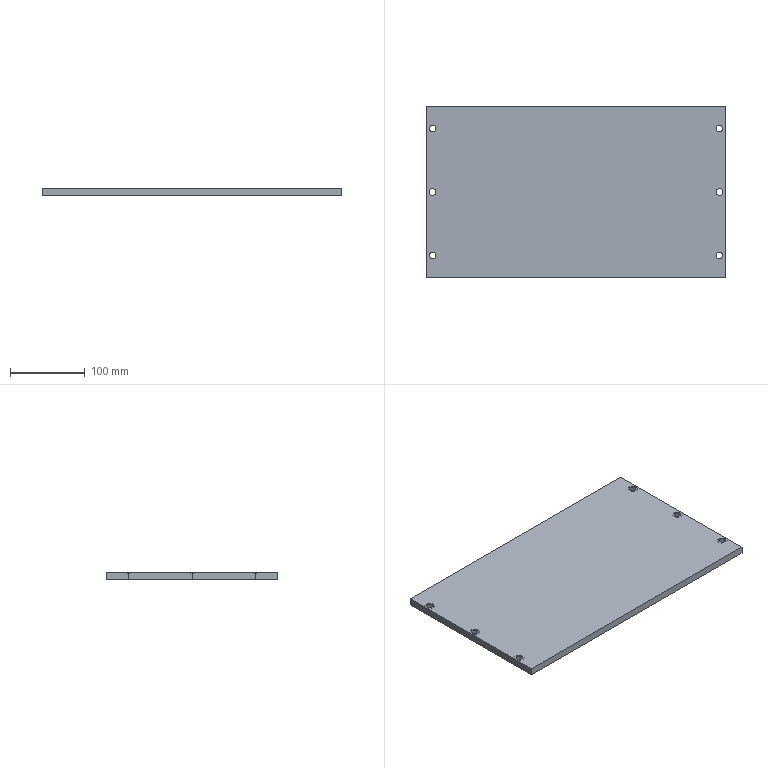Part | SolidWorks | features Cut 2, Extrusion 1, MirrorPattern 1 | 1 solid | 36 faces | box 400 x 230 x 10 mm | volume 912451 mm3 | cylinder 24 | plane 12 | commonest cylinder face diameters 9 x12 13 x12
STEP:
#1=CARTESIAN_POINT('',(186.,85.,9.));
#2=VERTEX_POINT('',#1);
#3=CARTESIAN_POINT('',(199.,85.,9.));
#4=VERTEX_POINT('',#3);
#5=CARTESIAN_POINT('',(192.5,85.,9.));
#6=DIRECTION('',(0.,0.,1.));
#7=DIRECTION('',(1.,0.,0.));
#8=AXIS2_PLACEMENT_3D('',#5,#6,#7);
#9=CIRCLE('',#8,6.5);
#10=EDGE_CURVE('',#2,#4,#9,.T.);
#11=ORIENTED_EDGE('',*,*,#10,.T.);
#12=CARTESIAN_POINT('',(199.,85.,0.));
#13=VERTEX_POINT('',#12);
#14=CARTESIAN_POINT('',(199.,85.,9.));
#15=DIRECTION('',(0.,0.,-1.));
#16=VECTOR('',#15,1000.);
#17=LINE('',#14,#16);
#18=EDGE_CURVE('',#4,#13,#17,.T.);
#19=ORIENTED_EDGE('',*,*,#18,.T.);
#20=CARTESIAN_POINT('',(186.,85.,0.));
#21=VERTEX_POINT('',#20);
#22=CARTESIAN_POINT('',(192.5,85.,0.));
#23=DIRECTION('',(0.,0.,1.));
#24=DIRECTION('',(1.,0.,0.));
#25=AXIS2_PLACEMENT_3D('',#22,#23,#24);
#26=CIRCLE('',#25,6.5);
#27=EDGE_CURVE('',#21,#13,#26,.T.);
#28=ORIENTED_EDGE('',*,*,#27,.F.);
#29=CARTESIAN_POINT('',(186.,85.,9.));
#30=DIRECTION('',(0.,0.,-1.));
#31=VECTOR('',#30,1000.);
#32=LINE('',#29,#31);
#33=EDGE_CURVE('',#2,#21,#32,.T.);
#34=ORIENTED_EDGE('',*,*,#33,.F.);
#35=EDGE_LOOP('',(#11,#19,#28,#34));
#36=FACE_OUTER_BOUND('',#35,.T.);
#37=CARTESIAN_POINT('',(192.5,85.,9.));
#38=DIRECTION('',(0.,0.,-1.));
#39=DIRECTION('',(-1.,0.,0.));
#40=AXIS2_PLACEMENT_3D('',#37,#38,#39);
#41=CYLINDRICAL_SURFACE('',#40,6.5);
#42=ADVANCED_FACE('',(#36),#41,.F.);
#43=CARTESIAN_POINT('',(186.,0.,9.));
#44=VERTEX_POINT('',#43);
#45=CARTESIAN_POINT('',(199.,0.,9.));
#46=VERTEX_POINT('',#45);
#47=CARTESIAN_POINT('',(192.5,0.,9.));
#48=DIRECTION('',(0.,0.,1.));
#49=DIRECTION('',(1.,0.,0.));
#50=AXIS2_PLACEMENT_3D('',#47,#48,#49);
#51=CIRCLE('',#50,6.5);
#52=EDGE_CURVE('',#44,#46,#51,.T.);
#53=ORIENTED_EDGE('',*,*,#52,.T.);
#54=CARTESIAN_POINT('',(199.,0.,0.));
#55=VERTEX_POINT('',#54);
#56=CARTESIAN_POINT('',(199.,0.,9.));
#57=DIRECTION('',(0.,0.,-1.));
#58=VECTOR('',#57,1000.);
#59=LINE('',#56,#58);
#60=EDGE_CURVE('',#46,#55,#59,.T.);
#61=ORIENTED_EDGE('',*,*,#60,.T.);
#62=CARTESIAN_POINT('',(186.,0.,0.));
#63=VERTEX_POINT('',#62);
#64=CARTESIAN_POINT('',(192.5,0.,0.));
#65=DIRECTION('',(0.,0.,1.));
#66=DIRECTION('',(1.,0.,0.));
#67=AXIS2_PLACEMENT_3D('',#64,#65,#66);
#68=CIRCLE('',#67,6.5);
#69=EDGE_CURVE('',#63,#55,#68,.T.);
#70=ORIENTED_EDGE('',*,*,#69,.F.);
#71=CARTESIAN_POINT('',(186.,0.,9.));
#72=DIRECTION('',(0.,0.,-1.));
#73=VECTOR('',#72,1000.);
#74=LINE('',#71,#73);
#75=EDGE_CURVE('',#44,#63,#74,.T.);
#76=ORIENTED_EDGE('',*,*,#75,.F.);
#77=EDGE_LOOP('',(#53,#61,#70,#76));
#78=FACE_OUTER_BOUND('',#77,.T.);
#79=CARTESIAN_POINT('',(192.5,0.,9.));
#80=DIRECTION('',(0.,0.,-1.));
#81=DIRECTION('',(-1.,0.,0.));
#82=AXIS2_PLACEMENT_3D('',#79,#80,#81);
#83=CYLINDRICAL_SURFACE('',#82,6.5);
#84=ADVANCED_FACE('',(#78),#83,.F.);
#85=CARTESIAN_POINT('',(186.,-85.,9.));
#86=VERTEX_POINT('',#85);
#87=CARTESIAN_POINT('',(199.,-85.,9.));
#88=VERTEX_POINT('',#87);
#89=CARTESIAN_POINT('',(192.5,-85.,9.));
#90=DIRECTION('',(0.,0.,1.));
#91=DIRECTION('',(1.,0.,0.));
#92=AXIS2_PLACEMENT_3D('',#89,#90,#91);
#93=CIRCLE('',#92,6.5);
#94=EDGE_CURVE('',#86,#88,#93,.T.);
#95=ORIENTED_EDGE('',*,*,#94,.T.);
#96=CARTESIAN_POINT('',(199.,-85.,0.));
#97=VERTEX_POINT('',#96);
#98=CARTESIAN_POINT('',(199.,-85.,9.));
#99=DIRECTION('',(0.,0.,-1.));
#100=VECTOR('',#99,1000.);
#101=LINE('',#98,#100);
#102=EDGE_CURVE('',#88,#97,#101,.T.);
#103=ORIENTED_EDGE('',*,*,#102,.T.);
#104=CARTESIAN_POINT('',(186.,-85.,0.));
#105=VERTEX_POINT('',#104);
#106=CARTESIAN_POINT('',(192.5,-85.,0.));
#107=DIRECTION('',(0.,0.,1.));
#108=DIRECTION('',(1.,0.,0.));
#109=AXIS2_PLACEMENT_3D('',#106,#107,#108);
#110=CIRCLE('',#109,6.5);
#111=EDGE_CURVE('',#105,#97,#110,.T.);
#112=ORIENTED_EDGE('',*,*,#111,.F.);
#113=CARTESIAN_POINT('',(186.,-85.,9.));
#114=DIRECTION('',(0.,0.,-1.));
#115=VECTOR('',#114,1000.);
#116=LINE('',#113,#115);
#117=EDGE_CURVE('',#86,#105,#116,.T.);
#118=ORIENTED_EDGE('',*,*,#117,.F.);
#119=EDGE_LOOP('',(#95,#103,#112,#118));
#120=FACE_OUTER_BOUND('',#119,.T.);
#121=CARTESIAN_POINT('',(192.5,-85.,9.));
#122=DIRECTION('',(0.,0.,-1.));
#123=DIRECTION('',(-1.,0.,0.));
#124=AXIS2_PLACEMENT_3D('',#121,#122,#123);
#125=CYLINDRICAL_SURFACE('',#124,6.5);
#126=ADVANCED_FACE('',(#120),#125,.F.);
#127=CARTESIAN_POINT('',(-186.,85.,9.));
#128=VERTEX_POINT('',#127);
#129=CARTESIAN_POINT('',(-199.,85.,9.));
#130=VERTEX_POINT('',#129);
#131=CARTESIAN_POINT('',(-192.5,85.,9.));
#132=DIRECTION('',(0.,0.,-1.));
#133=DIRECTION('',(-1.,0.,0.));
#134=AXIS2_PLACEMENT_3D('',#131,#132,#133);
#135=CIRCLE('',#134,6.5);
#136=EDGE_CURVE('',#128,#130,#135,.T.);
#137=ORIENTED_EDGE('',*,*,#136,.F.);
#138=CARTESIAN_POINT('',(-186.,85.,0.));
#139=VERTEX_POINT('',#138);
#140=CARTESIAN_POINT('',(-186.,85.,9.));
#141=DIRECTION('',(0.,0.,-1.));
#142=VECTOR('',#141,1000.);
#143=LINE('',#140,#142);
#144=EDGE_CURVE('',#128,#139,#143,.T.);
#145=ORIENTED_EDGE('',*,*,#144,.T.);
#146=CARTESIAN_POINT('',(-199.,85.,0.));
#147=VERTEX_POINT('',#146);
#148=CARTESIAN_POINT('',(-192.5,85.,0.));
#149=DIRECTION('',(0.,0.,-1.));
#150=DIRECTION('',(-1.,0.,0.));
#151=AXIS2_PLACEMENT_3D('',#148,#149,#150);
#152=CIRCLE('',#151,6.5);
#153=EDGE_CURVE('',#139,#147,#152,.T.);
#154=ORIENTED_EDGE('',*,*,#153,.T.);
#155=CARTESIAN_POINT('',(-199.,85.,9.));
#156=DIRECTION('',(0.,0.,-1.));
#157=VECTOR('',#156,1000.);
#158=LINE('',#155,#157);
#159=EDGE_CURVE('',#130,#147,#158,.T.);
#160=ORIENTED_EDGE('',*,*,#159,.F.);
#161=EDGE_LOOP('',(#137,#145,#154,#160));
#162=FACE_OUTER_BOUND('',#161,.T.);
#163=CARTESIAN_POINT('',(-192.5,85.,9.));
#164=DIRECTION('',(0.,0.,-1.));
#165=DIRECTION('',(-1.,0.,0.));
#166=AXIS2_PLACEMENT_3D('',#163,#164,#165);
#167=CYLINDRICAL_SURFACE('',#166,6.5);
#168=ADVANCED_FACE('',(#162),#167,.F.);
#169=CARTESIAN_POINT('',(-186.,0.,9.));
#170=VERTEX_POINT('',#169);
#171=CARTESIAN_POINT('',(-199.,0.,9.));
#172=VERTEX_POINT('',#171);
#173=CARTESIAN_POINT('',(-192.5,0.,9.));
#174=DIRECTION('',(0.,0.,-1.));
#175=DIRECTION('',(-1.,0.,0.));
#176=AXIS2_PLACEMENT_3D('',#173,#174,#175);
#177=CIRCLE('',#176,6.5);
#178=EDGE_CURVE('',#170,#172,#177,.T.);
#179=ORIENTED_EDGE('',*,*,#178,.F.);
#180=CARTESIAN_POINT('',(-186.,0.,0.));
#181=VERTEX_POINT('',#180);
#182=CARTESIAN_POINT('',(-186.,0.,9.));
#183=DIRECTION('',(0.,0.,-1.));
#184=VECTOR('',#183,1000.);
#185=LINE('',#182,#184);
#186=EDGE_CURVE('',#170,#181,#185,.T.);
#187=ORIENTED_EDGE('',*,*,#186,.T.);
#188=CARTESIAN_POINT('',(-199.,0.,0.));
#189=VERTEX_POINT('',#188);
#190=CARTESIAN_POINT('',(-192.5,0.,0.));
#191=DIRECTION('',(0.,0.,-1.));
#192=DIRECTION('',(-1.,0.,0.));
#193=AXIS2_PLACEMENT_3D('',#190,#191,#192);
#194=CIRCLE('',#193,6.5);
#195=EDGE_CURVE('',#181,#189,#194,.T.);
#196=ORIENTED_EDGE('',*,*,#195,.T.);
#197=CARTESIAN_POINT('',(-199.,0.,9.));
#198=DIRECTION('',(0.,0.,-1.));
#199=VECTOR('',#198,1000.);
#200=LINE('',#197,#199);
#201=EDGE_CURVE('',#172,#189,#200,.T.);
#202=ORIENTED_EDGE('',*,*,#201,.F.);
#203=EDGE_LOOP('',(#179,#187,#196,#202));
#204=FACE_OUTER_BOUND('',#203,.T.);
#205=CARTESIAN_POINT('',(-192.5,0.,9.));
#206=DIRECTION('',(0.,0.,-1.));
#207=DIRECTION('',(-1.,0.,0.));
#208=AXIS2_PLACEMENT_3D('',#205,#206,#207);
#209=CYLINDRICAL_SURFACE('',#208,6.5);
#210=ADVANCED_FACE('',(#204),#209,.F.);
#211=CARTESIAN_POINT('',(-186.,-85.,9.));
#212=VERTEX_POINT('',#211);
#213=CARTESIAN_POINT('',(-199.,-85.,9.));
#214=VERTEX_POINT('',#213);
#215=CARTESIAN_POINT('',(-192.5,-85.,9.));
#216=DIRECTION('',(0.,0.,-1.));
#217=DIRECTION('',(-1.,0.,0.));
#218=AXIS2_PLACEMENT_3D('',#215,#216,#217);
#219=CIRCLE('',#218,6.5);
#220=EDGE_CURVE('',#212,#214,#219,.T.);
#221=ORIENTED_EDGE('',*,*,#220,.F.);
#222=CARTESIAN_POINT('',(-186.,-85.,0.));
#223=VERTEX_POINT('',#222);
#224=CARTESIAN_POINT('',(-186.,-85.,9.));
#225=DIRECTION('',(0.,0.,-1.));
#226=VECTOR('',#225,1000.);
#227=LINE('',#224,#226);
#228=EDGE_CURVE('',#212,#223,#227,.T.);
#229=ORIENTED_EDGE('',*,*,#228,.T.);
#230=CARTESIAN_POINT('',(-199.,-85.,0.));
#231=VERTEX_POINT('',#230);
#232=CARTESIAN_POINT('',(-192.5,-85.,0.));
#233=DIRECTION('',(0.,0.,-1.));
#234=DIRECTION('',(-1.,0.,0.));
#235=AXIS2_PLACEMENT_3D('',#232,#233,#234);
#236=CIRCLE('',#235,6.5);
#237=EDGE_CURVE('',#223,#231,#236,.T.);
#238=ORIENTED_EDGE('',*,*,#237,.T.);
#239=CARTESIAN_POINT('',(-199.,-85.,9.));
#240=DIRECTION('',(0.,0.,-1.));
#241=VECTOR('',#240,1000.);
#242=LINE('',#239,#241);
#243=EDGE_CURVE('',#214,#231,#242,.T.);
#244=ORIENTED_EDGE('',*,*,#243,.F.);
#245=EDGE_LOOP('',(#221,#229,#238,#244));
#246=FACE_OUTER_BOUND('',#245,.T.);
#247=CARTESIAN_POINT('',(-192.5,-85.,9.));
#248=DIRECTION('',(0.,0.,-1.));
#249=DIRECTION('',(-1.,0.,0.));
#250=AXIS2_PLACEMENT_3D('',#247,#248,#249);
#251=CYLINDRICAL_SURFACE('',#250,6.5);
#252=ADVANCED_FACE('',(#246),#251,.F.);
#253=CARTESIAN_POINT('',(-197.,-85.,10.));
#254=VERTEX_POINT('',#253);
#255=CARTESIAN_POINT('',(-188.,-85.,10.));
#256=VERTEX_POINT('',#255);
#257=CARTESIAN_POINT('',(-192.5,-85.,10.));
#258=DIRECTION('',(0.,0.,1.));
#259=DIRECTION('',(1.,0.,0.));
#260=AXIS2_PLACEMENT_3D('',#257,#258,#259);
#261=CIRCLE('',#260,4.5);
#262=EDGE_CURVE('',#254,#256,#261,.T.);
#263=ORIENTED_EDGE('',*,*,#262,.T.);
#264=CARTESIAN_POINT('',(-188.,-85.,9.));
#265=VERTEX_POINT('',#264);
#266=CARTESIAN_POINT('',(-188.,-85.,25.));
#267=DIRECTION('',(0.,0.,-1.));
#268=VECTOR('',#267,1000.);
#269=LINE('',#266,#268);
#270=EDGE_CURVE('',#256,#265,#269,.T.);
#271=ORIENTED_EDGE('',*,*,#270,.T.);
#272=CARTESIAN_POINT('',(-197.,-85.,9.));
#273=VERTEX_POINT('',#272);
#274=CARTESIAN_POINT('',(-192.5,-85.,9.));
#275=DIRECTION('',(0.,0.,1.));
#276=DIRECTION('',(-1.,0.,0.));
#277=AXIS2_PLACEMENT_3D('',#274,#275,#276);
#278=CIRCLE('',#277,4.5);
#279=EDGE_CURVE('',#273,#265,#278,.T.);
#280=ORIENTED_EDGE('',*,*,#279,.F.);
#281=CARTESIAN_POINT('',(-197.,-85.,25.));
#282=DIRECTION('',(0.,0.,-1.));
#283=VECTOR('',#282,1000.);
#284=LINE('',#281,#283);
#285=EDGE_CURVE('',#254,#273,#284,.T.);
#286=ORIENTED_EDGE('',*,*,#285,.F.);
#287=EDGE_LOOP('',(#263,#271,#280,#286));
#288=FACE_OUTER_BOUND('',#287,.T.);
#289=CARTESIAN_POINT('',(-192.5,-85.,25.));
#290=DIRECTION('',(0.,0.,-1.));
#291=DIRECTION('',(-1.,0.,0.));
#292=AXIS2_PLACEMENT_3D('',#289,#290,#291);
#293=CYLINDRICAL_SURFACE('',#292,4.5);
#294=ADVANCED_FACE('',(#288),#293,.F.);
#295=CARTESIAN_POINT('',(-197.,0.,10.));
#296=VERTEX_POINT('',#295);
#297=CARTESIAN_POINT('',(-188.,0.,10.));
#298=VERTEX_POINT('',#297);
#299=CARTESIAN_POINT('',(-192.5,0.,10.));
#300=DIRECTION('',(0.,0.,1.));
#301=DIRECTION('',(1.,0.,0.));
#302=AXIS2_PLACEMENT_3D('',#299,#300,#301);
#303=CIRCLE('',#302,4.5);
#304=EDGE_CURVE('',#296,#298,#303,.T.);
#305=ORIENTED_EDGE('',*,*,#304,.T.);
#306=CARTESIAN_POINT('',(-188.,0.,9.));
#307=VERTEX_POINT('',#306);
#308=CARTESIAN_POINT('',(-188.,0.,25.));
#309=DIRECTION('',(0.,0.,-1.));
#310=VECTOR('',#309,1000.);
#311=LINE('',#308,#310);
#312=EDGE_CURVE('',#298,#307,#311,.T.);
#313=ORIENTED_EDGE('',*,*,#312,.T.);
#314=CARTESIAN_POINT('',(-197.,0.,9.));
#315=VERTEX_POINT('',#314);
#316=CARTESIAN_POINT('',(-192.5,0.,9.));
#317=DIRECTION('',(0.,0.,1.));
#318=DIRECTION('',(-1.,0.,0.));
#319=AXIS2_PLACEMENT_3D('',#316,#317,#318);
#320=CIRCLE('',#319,4.5);
#321=EDGE_CURVE('',#315,#307,#320,.T.);
#322=ORIENTED_EDGE('',*,*,#321,.F.);
#323=CARTESIAN_POINT('',(-197.,0.,25.));
#324=DIRECTION('',(0.,0.,-1.));
#325=VECTOR('',#324,1000.);
#326=LINE('',#323,#325);
#327=EDGE_CURVE('',#296,#315,#326,.T.);
#328=ORIENTED_EDGE('',*,*,#327,.F.);
#329=EDGE_LOOP('',(#305,#313,#322,#328));
#330=FACE_OUTER_BOUND('',#329,.T.);
#331=CARTESIAN_POINT('',(-192.5,0.,25.));
#332=DIRECTION('',(0.,0.,-1.));
#333=DIRECTION('',(-1.,0.,0.));
#334=AXIS2_PLACEMENT_3D('',#331,#332,#333);
#335=CYLINDRICAL_SURFACE('',#334,4.5);
#336=ADVANCED_FACE('',(#330),#335,.F.);
#337=CARTESIAN_POINT('',(-197.,85.,10.));
#338=VERTEX_POINT('',#337);
#339=CARTESIAN_POINT('',(-188.,85.,10.));
#340=VERTEX_POINT('',#339);
#341=CARTESIAN_POINT('',(-192.5,85.,10.));
#342=DIRECTION('',(0.,0.,1.));
#343=DIRECTION('',(1.,0.,0.));
#344=AXIS2_PLACEMENT_3D('',#341,#342,#343);
#345=CIRCLE('',#344,4.5);
#346=EDGE_CURVE('',#338,#340,#345,.T.);
#347=ORIENTED_EDGE('',*,*,#346,.T.);
#348=CARTESIAN_POINT('',(-188.,85.,9.));
#349=VERTEX_POINT('',#348);
#350=CARTESIAN_POINT('',(-188.,85.,25.));
#351=DIRECTION('',(0.,0.,-1.));
#352=VECTOR('',#351,1000.);
#353=LINE('',#350,#352);
#354=EDGE_CURVE('',#340,#349,#353,.T.);
#355=ORIENTED_EDGE('',*,*,#354,.T.);
#356=CARTESIAN_POINT('',(-197.,85.,9.));
#357=VERTEX_POINT('',#356);
#358=CARTESIAN_POINT('',(-192.5,85.,9.));
#359=DIRECTION('',(0.,0.,1.));
#360=DIRECTION('',(-1.,0.,0.));
#361=AXIS2_PLACEMENT_3D('',#358,#359,#360);
#362=CIRCLE('',#361,4.5);
#363=EDGE_CURVE('',#357,#349,#362,.T.);
#364=ORIENTED_EDGE('',*,*,#363,.F.);
#365=CARTESIAN_POINT('',(-197.,85.,25.));
#366=DIRECTION('',(0.,0.,-1.));
#367=VECTOR('',#366,1000.);
#368=LINE('',#365,#367);
#369=EDGE_CURVE('',#338,#357,#368,.T.);
#370=ORIENTED_EDGE('',*,*,#369,.F.);
#371=EDGE_LOOP('',(#347,#355,#364,#370));
#372=FACE_OUTER_BOUND('',#371,.T.);
#373=CARTESIAN_POINT('',(-192.5,85.,25.));
#374=DIRECTION('',(0.,0.,-1.));
#375=DIRECTION('',(-1.,0.,0.));
#376=AXIS2_PLACEMENT_3D('',#373,#374,#375);
#377=CYLINDRICAL_SURFACE('',#376,4.5);
#378=ADVANCED_FACE('',(#372),#377,.F.);
#379=CARTESIAN_POINT('',(197.,-85.,10.));
#380=VERTEX_POINT('',#379);
#381=CARTESIAN_POINT('',(188.,-85.,10.));
#382=VERTEX_POINT('',#381);
#383=CARTESIAN_POINT('',(192.5,-85.,10.));
#384=DIRECTION('',(0.,0.,-1.));
#385=DIRECTION('',(1.,0.,0.));
#386=AXIS2_PLACEMENT_3D('',#383,#384,#385);
#387=CIRCLE('',#386,4.5);
#388=EDGE_CURVE('',#380,#382,#387,.T.);
#389=ORIENTED_EDGE('',*,*,#388,.F.);
#390=CARTESIAN_POINT('',(197.,-85.,9.));
#391=VERTEX_POINT('',#390);
#392=CARTESIAN_POINT('',(197.,-85.,25.));
#393=DIRECTION('',(0.,0.,-1.));
#394=VECTOR('',#393,1000.);
#395=LINE('',#392,#394);
#396=EDGE_CURVE('',#380,#391,#395,.T.);
#397=ORIENTED_EDGE('',*,*,#396,.T.);
#398=CARTESIAN_POINT('',(188.,-85.,9.));
#399=VERTEX_POINT('',#398);
#400=CARTESIAN_POINT('',(192.5,-85.,9.));
#401=DIRECTION('',(0.,0.,-1.));
#402=DIRECTION('',(-1.,0.,0.));
#403=AXIS2_PLACEMENT_3D('',#400,#401,#402);
#404=CIRCLE('',#403,4.5);
#405=EDGE_CURVE('',#391,#399,#404,.T.);
#406=ORIENTED_EDGE('',*,*,#405,.T.);
#407=CARTESIAN_POINT('',(188.,-85.,25.));
#408=DIRECTION('',(0.,0.,-1.));
#409=VECTOR('',#408,1000.);
#410=LINE('',#407,#409);
#411=EDGE_CURVE('',#382,#399,#410,.T.);
#412=ORIENTED_EDGE('',*,*,#411,.F.);
#413=EDGE_LOOP('',(#389,#397,#406,#412));
#414=FACE_OUTER_BOUND('',#413,.T.);
#415=CARTESIAN_POINT('',(192.5,-85.,25.));
#416=DIRECTION('',(0.,0.,-1.));
#417=DIRECTION('',(-1.,0.,0.));
#418=AXIS2_PLACEMENT_3D('',#415,#416,#417);
#419=CYLINDRICAL_SURFACE('',#418,4.5);
#420=ADVANCED_FACE('',(#414),#419,.F.);
#421=CARTESIAN_POINT('',(197.,0.,10.));
#422=VERTEX_POINT('',#421);
#423=CARTESIAN_POINT('',(188.,0.,10.));
#424=VERTEX_POINT('',#423);
#425=CARTESIAN_POINT('',(192.5,0.,10.));
#426=DIRECTION('',(0.,0.,-1.));
#427=DIRECTION('',(1.,0.,0.));
#428=AXIS2_PLACEMENT_3D('',#425,#426,#427);
#429=CIRCLE('',#428,4.5);
#430=EDGE_CURVE('',#422,#424,#429,.T.);
#431=ORIENTED_EDGE('',*,*,#430,.F.);
#432=CARTESIAN_POINT('',(197.,0.,9.));
#433=VERTEX_POINT('',#432);
#434=CARTESIAN_POINT('',(197.,0.,25.));
#435=DIRECTION('',(0.,0.,-1.));
#436=VECTOR('',#435,1000.);
#437=LINE('',#434,#436);
#438=EDGE_CURVE('',#422,#433,#437,.T.);
#439=ORIENTED_EDGE('',*,*,#438,.T.);
#440=CARTESIAN_POINT('',(188.,0.,9.));
#441=VERTEX_POINT('',#440);
#442=CARTESIAN_POINT('',(192.5,0.,9.));
#443=DIRECTION('',(0.,0.,-1.));
#444=DIRECTION('',(-1.,0.,0.));
#445=AXIS2_PLACEMENT_3D('',#442,#443,#444);
#446=CIRCLE('',#445,4.5);
#447=EDGE_CURVE('',#433,#441,#446,.T.);
#448=ORIENTED_EDGE('',*,*,#447,.T.);
#449=CARTESIAN_POINT('',(188.,0.,25.));
#450=DIRECTION('',(0.,0.,-1.));
#451=VECTOR('',#450,1000.);
#452=LINE('',#449,#451);
#453=EDGE_CURVE('',#424,#441,#452,.T.);
#454=ORIENTED_EDGE('',*,*,#453,.F.);
#455=EDGE_LOOP('',(#431,#439,#448,#454));
#456=FACE_OUTER_BOUND('',#455,.T.);
#457=CARTESIAN_POINT('',(192.5,0.,25.));
#458=DIRECTION('',(0.,0.,-1.));
#459=DIRECTION('',(-1.,0.,0.));
#460=AXIS2_PLACEMENT_3D('',#457,#458,#459);
#461=CYLINDRICAL_SURFACE('',#460,4.5);
#462=ADVANCED_FACE('',(#456),#461,.F.);
#463=CARTESIAN_POINT('',(197.,85.,10.));
#464=VERTEX_POINT('',#463);
#465=CARTESIAN_POINT('',(188.,85.,10.));
#466=VERTEX_POINT('',#465);
#467=CARTESIAN_POINT('',(192.5,85.,10.));
#468=DIRECTION('',(0.,0.,-1.));
#469=DIRECTION('',(1.,0.,0.));
#470=AXIS2_PLACEMENT_3D('',#467,#468,#469);
#471=CIRCLE('',#470,4.5);
#472=EDGE_CURVE('',#464,#466,#471,.T.);
#473=ORIENTED_EDGE('',*,*,#472,.F.);
#474=CARTESIAN_POINT('',(197.,85.,9.));
#475=VERTEX_POINT('',#474);
#476=CARTESIAN_POINT('',(197.,85.,25.));
#477=DIRECTION('',(0.,0.,-1.));
#478=VECTOR('',#477,1000.);
#479=LINE('',#476,#478);
#480=EDGE_CURVE('',#464,#475,#479,.T.);
#481=ORIENTED_EDGE('',*,*,#480,.T.);
#482=CARTESIAN_POINT('',(188.,85.,9.));
#483=VERTEX_POINT('',#482);
#484=CARTESIAN_POINT('',(192.5,85.,9.));
#485=DIRECTION('',(0.,0.,-1.));
#486=DIRECTION('',(-1.,0.,0.));
#487=AXIS2_PLACEMENT_3D('',#484,#485,#486);
#488=CIRCLE('',#487,4.5);
#489=EDGE_CURVE('',#475,#483,#488,.T.);
#490=ORIENTED_EDGE('',*,*,#489,.T.);
#491=CARTESIAN_POINT('',(188.,85.,25.));
#492=DIRECTION('',(0.,0.,-1.));
#493=VECTOR('',#492,1000.);
#494=LINE('',#491,#493);
#495=EDGE_CURVE('',#466,#483,#494,.T.);
#496=ORIENTED_EDGE('',*,*,#495,.F.);
#497=EDGE_LOOP('',(#473,#481,#490,#496));
#498=FACE_OUTER_BOUND('',#497,.T.);
#499=CARTESIAN_POINT('',(192.5,85.,25.));
#500=DIRECTION('',(0.,0.,-1.));
#501=DIRECTION('',(-1.,0.,0.));
#502=AXIS2_PLACEMENT_3D('',#499,#500,#501);
#503=CYLINDRICAL_SURFACE('',#502,4.5);
#504=ADVANCED_FACE('',(#498),#503,.F.);
#505=ORIENTED_EDGE('',*,*,#69,.T.);
#506=CARTESIAN_POINT('',(192.5,0.,0.));
#507=DIRECTION('',(0.,0.,1.));
#508=DIRECTION('',(1.,0.,0.));
#509=AXIS2_PLACEMENT_3D('',#506,#507,#508);
#510=CIRCLE('',#509,6.5);
#511=EDGE_CURVE('',#55,#63,#510,.T.);
#512=ORIENTED_EDGE('',*,*,#511,.T.);
#513=EDGE_LOOP('',(#505,#512));
#514=FACE_BOUND('',#513,.T.);
#515=CARTESIAN_POINT('',(-192.5,85.,0.));
#516=DIRECTION('',(0.,0.,-1.));
#517=DIRECTION('',(-1.,0.,0.));
#518=AXIS2_PLACEMENT_3D('',#515,#516,#517);
#519=CIRCLE('',#518,6.5);
#520=EDGE_CURVE('',#147,#139,#519,.T.);
#521=ORIENTED_EDGE('',*,*,#520,.F.);
#522=ORIENTED_EDGE('',*,*,#153,.F.);
#523=EDGE_LOOP('',(#521,#522));
#524=FACE_BOUND('',#523,.T.);
#525=CARTESIAN_POINT('',(-192.5,0.,0.));
#526=DIRECTION('',(0.,0.,-1.));
#527=DIRECTION('',(-1.,0.,0.));
#528=AXIS2_PLACEMENT_3D('',#525,#526,#527);
#529=CIRCLE('',#528,6.5);
#530=EDGE_CURVE('',#189,#181,#529,.T.);
#531=ORIENTED_EDGE('',*,*,#530,.F.);
#532=ORIENTED_EDGE('',*,*,#195,.F.);
#533=EDGE_LOOP('',(#531,#532));
#534=FACE_BOUND('',#533,.T.);
#535=CARTESIAN_POINT('',(-192.5,-85.,0.));
#536=DIRECTION('',(0.,0.,-1.));
#537=DIRECTION('',(-1.,0.,0.));
#538=AXIS2_PLACEMENT_3D('',#535,#536,#537);
#539=CIRCLE('',#538,6.5);
#540=EDGE_CURVE('',#231,#223,#539,.T.);
#541=ORIENTED_EDGE('',*,*,#540,.F.);
#542=ORIENTED_EDGE('',*,*,#237,.F.);
#543=EDGE_LOOP('',(#541,#542));
#544=FACE_BOUND('',#543,.T.);
#545=CARTESIAN_POINT('',(-200.,115.,0.));
#546=VERTEX_POINT('',#545);
#547=CARTESIAN_POINT('',(-200.,-115.,0.));
#548=VERTEX_POINT('',#547);
#549=CARTESIAN_POINT('',(-200.,-115.,0.));
#550=DIRECTION('',(0.,-1.,0.));
#551=VECTOR('',#550,1000.);
#552=LINE('',#549,#551);
#553=EDGE_CURVE('',#546,#548,#552,.T.);
#554=ORIENTED_EDGE('',*,*,#553,.F.);
#555=CARTESIAN_POINT('',(200.,115.,0.));
#556=VERTEX_POINT('',#555);
#557=CARTESIAN_POINT('',(200.,115.,0.));
#558=DIRECTION('',(-1.,0.,0.));
#559=VECTOR('',#558,1000.);
#560=LINE('',#557,#559);
#561=EDGE_CURVE('',#556,#546,#560,.T.);
#562=ORIENTED_EDGE('',*,*,#561,.F.);
#563=CARTESIAN_POINT('',(200.,-115.,0.));
#564=VERTEX_POINT('',#563);
#565=CARTESIAN_POINT('',(200.,-115.,0.));
#566=DIRECTION('',(0.,1.,0.));
#567=VECTOR('',#566,1000.);
#568=LINE('',#565,#567);
#569=EDGE_CURVE('',#564,#556,#568,.T.);
#570=ORIENTED_EDGE('',*,*,#569,.F.);
#571=CARTESIAN_POINT('',(200.,-115.,0.));
#572=DIRECTION('',(1.,0.,0.));
#573=VECTOR('',#572,1000.);
#574=LINE('',#571,#573);
#575=EDGE_CURVE('',#548,#564,#574,.T.);
#576=ORIENTED_EDGE('',*,*,#575,.F.);
#577=EDGE_LOOP('',(#554,#562,#570,#576));
#578=FACE_OUTER_BOUND('',#577,.T.);
#579=ORIENTED_EDGE('',*,*,#111,.T.);
#580=CARTESIAN_POINT('',(192.5,-85.,0.));
#581=DIRECTION('',(0.,0.,1.));
#582=DIRECTION('',(1.,0.,0.));
#583=AXIS2_PLACEMENT_3D('',#580,#581,#582);
#584=CIRCLE('',#583,6.5);
#585=EDGE_CURVE('',#97,#105,#584,.T.);
#586=ORIENTED_EDGE('',*,*,#585,.T.);
#587=EDGE_LOOP('',(#579,#586));
#588=FACE_BOUND('',#587,.T.);
#589=ORIENTED_EDGE('',*,*,#27,.T.);
#590=CARTESIAN_POINT('',(192.5,85.,0.));
#591=DIRECTION('',(0.,0.,1.));
#592=DIRECTION('',(1.,0.,0.));
#593=AXIS2_PLACEMENT_3D('',#590,#591,#592);
#594=CIRCLE('',#593,6.5);
#595=EDGE_CURVE('',#13,#21,#594,.T.);
#596=ORIENTED_EDGE('',*,*,#595,.T.);
#597=EDGE_LOOP('',(#589,#596));
#598=FACE_BOUND('',#597,.T.);
#599=CARTESIAN_POINT('',(0.,0.,0.));
#600=DIRECTION('',(0.,0.,1.));
#601=DIRECTION('',(1.,0.,0.));
#602=AXIS2_PLACEMENT_3D('',#599,#600,#601);
#603=PLANE('',#602);
#604=ADVANCED_FACE('',(#514,#524,#534,#544,#578,#588,#598),#603,.F.);
#605=ORIENTED_EDGE('',*,*,#480,.F.);
#606=CARTESIAN_POINT('',(192.5,85.,10.));
#607=DIRECTION('',(0.,0.,-1.));
#608=DIRECTION('',(1.,0.,0.));
#609=AXIS2_PLACEMENT_3D('',#606,#607,#608);
#610=CIRCLE('',#609,4.5);
#611=EDGE_CURVE('',#466,#464,#610,.T.);
#612=ORIENTED_EDGE('',*,*,#611,.F.);
#613=ORIENTED_EDGE('',*,*,#495,.T.);
#614=CARTESIAN_POINT('',(192.5,85.,9.));
#615=DIRECTION('',(0.,0.,-1.));
#616=DIRECTION('',(-1.,0.,0.));
#617=AXIS2_PLACEMENT_3D('',#614,#615,#616);
#618=CIRCLE('',#617,4.5);
#619=EDGE_CURVE('',#483,#475,#618,.T.);
#620=ORIENTED_EDGE('',*,*,#619,.T.);
#621=EDGE_LOOP('',(#605,#612,#613,#620));
#622=FACE_OUTER_BOUND('',#621,.T.);
#623=CARTESIAN_POINT('',(192.5,85.,25.));
#624=DIRECTION('',(0.,0.,-1.));
#625=DIRECTION('',(-1.,0.,0.));
#626=AXIS2_PLACEMENT_3D('',#623,#624,#625);
#627=CYLINDRICAL_SURFACE('',#626,4.5);
#628=ADVANCED_FACE('',(#622),#627,.F.);
#629=ORIENTED_EDGE('',*,*,#438,.F.);
#630=CARTESIAN_POINT('',(192.5,0.,10.));
#631=DIRECTION('',(0.,0.,-1.));
#632=DIRECTION('',(1.,0.,0.));
#633=AXIS2_PLACEMENT_3D('',#630,#631,#632);
#634=CIRCLE('',#633,4.5);
#635=EDGE_CURVE('',#424,#422,#634,.T.);
#636=ORIENTED_EDGE('',*,*,#635,.F.);
#637=ORIENTED_EDGE('',*,*,#453,.T.);
#638=CARTESIAN_POINT('',(192.5,0.,9.));
#639=DIRECTION('',(0.,0.,-1.));
#640=DIRECTION('',(-1.,0.,0.));
#641=AXIS2_PLACEMENT_3D('',#638,#639,#640);
#642=CIRCLE('',#641,4.5);
#643=EDGE_CURVE('',#441,#433,#642,.T.);
#644=ORIENTED_EDGE('',*,*,#643,.T.);
#645=EDGE_LOOP('',(#629,#636,#637,#644));
#646=FACE_OUTER_BOUND('',#645,.T.);
#647=CARTESIAN_POINT('',(192.5,0.,25.));
#648=DIRECTION('',(0.,0.,-1.));
#649=DIRECTION('',(-1.,0.,0.));
#650=AXIS2_PLACEMENT_3D('',#647,#648,#649);
#651=CYLINDRICAL_SURFACE('',#650,4.5);
#652=ADVANCED_FACE('',(#646),#651,.F.);
#653=ORIENTED_EDGE('',*,*,#396,.F.);
#654=CARTESIAN_POINT('',(192.5,-85.,10.));
#655=DIRECTION('',(0.,0.,-1.));
#656=DIRECTION('',(1.,0.,0.));
#657=AXIS2_PLACEMENT_3D('',#654,#655,#656);
#658=CIRCLE('',#657,4.5);
#659=EDGE_CURVE('',#382,#380,#658,.T.);
#660=ORIENTED_EDGE('',*,*,#659,.F.);
#661=ORIENTED_EDGE('',*,*,#411,.T.);
#662=CARTESIAN_POINT('',(192.5,-85.,9.));
#663=DIRECTION('',(0.,0.,-1.));
#664=DIRECTION('',(-1.,0.,0.));
#665=AXIS2_PLACEMENT_3D('',#662,#663,#664);
#666=CIRCLE('',#665,4.5);
#667=EDGE_CURVE('',#399,#391,#666,.T.);
#668=ORIENTED_EDGE('',*,*,#667,.T.);
#669=EDGE_LOOP('',(#653,#660,#661,#668));
#670=FACE_OUTER_BOUND('',#669,.T.);
#671=CARTESIAN_POINT('',(192.5,-85.,25.));
#672=DIRECTION('',(0.,0.,-1.));
#673=DIRECTION('',(-1.,0.,0.));
#674=AXIS2_PLACEMENT_3D('',#671,#672,#673);
#675=CYLINDRICAL_SURFACE('',#674,4.5);
#676=ADVANCED_FACE('',(#670),#675,.F.);
#677=ORIENTED_EDGE('',*,*,#635,.T.);
#678=ORIENTED_EDGE('',*,*,#430,.T.);
#679=EDGE_LOOP('',(#677,#678));
#680=FACE_BOUND('',#679,.T.);
#681=CARTESIAN_POINT('',(-200.,115.,10.));
#682=VERTEX_POINT('',#681);
#683=CARTESIAN_POINT('',(-200.,-115.,10.));
#684=VERTEX_POINT('',#683);
#685=CARTESIAN_POINT('',(-200.,-115.,10.));
#686=DIRECTION('',(0.,-1.,0.));
#687=VECTOR('',#686,1000.);
#688=LINE('',#685,#687);
#689=EDGE_CURVE('',#682,#684,#688,.T.);
#690=ORIENTED_EDGE('',*,*,#689,.T.);
#691=CARTESIAN_POINT('',(200.,-115.,10.));
#692=VERTEX_POINT('',#691);
#693=CARTESIAN_POINT('',(200.,-115.,10.));
#694=DIRECTION('',(1.,0.,0.));
#695=VECTOR('',#694,1000.);
#696=LINE('',#693,#695);
#697=EDGE_CURVE('',#684,#692,#696,.T.);
#698=ORIENTED_EDGE('',*,*,#697,.T.);
#699=CARTESIAN_POINT('',(200.,115.,10.));
#700=VERTEX_POINT('',#699);
#701=CARTESIAN_POINT('',(200.,-115.,10.));
#702=DIRECTION('',(0.,1.,0.));
#703=VECTOR('',#702,1000.);
#704=LINE('',#701,#703);
#705=EDGE_CURVE('',#692,#700,#704,.T.);
#706=ORIENTED_EDGE('',*,*,#705,.T.);
#707=CARTESIAN_POINT('',(200.,115.,10.));
#708=DIRECTION('',(-1.,0.,0.));
#709=VECTOR('',#708,1000.);
#710=LINE('',#707,#709);
#711=EDGE_CURVE('',#700,#682,#710,.T.);
#712=ORIENTED_EDGE('',*,*,#711,.T.);
#713=EDGE_LOOP('',(#690,#698,#706,#712));
#714=FACE_OUTER_BOUND('',#713,.T.);
#715=ORIENTED_EDGE('',*,*,#262,.F.);
#716=CARTESIAN_POINT('',(-192.5,-85.,10.));
#717=DIRECTION('',(0.,0.,1.));
#718=DIRECTION('',(1.,0.,0.));
#719=AXIS2_PLACEMENT_3D('',#716,#717,#718);
#720=CIRCLE('',#719,4.5);
#721=EDGE_CURVE('',#256,#254,#720,.T.);
#722=ORIENTED_EDGE('',*,*,#721,.F.);
#723=EDGE_LOOP('',(#715,#722));
#724=FACE_BOUND('',#723,.T.);
#725=ORIENTED_EDGE('',*,*,#304,.F.);
#726=CARTESIAN_POINT('',(-192.5,0.,10.));
#727=DIRECTION('',(0.,0.,1.));
#728=DIRECTION('',(1.,0.,0.));
#729=AXIS2_PLACEMENT_3D('',#726,#727,#728);
#730=CIRCLE('',#729,4.5);
#731=EDGE_CURVE('',#298,#296,#730,.T.);
#732=ORIENTED_EDGE('',*,*,#731,.F.);
#733=EDGE_LOOP('',(#725,#732));
#734=FACE_BOUND('',#733,.T.);
#735=ORIENTED_EDGE('',*,*,#346,.F.);
#736=CARTESIAN_POINT('',(-192.5,85.,10.));
#737=DIRECTION('',(0.,0.,1.));
#738=DIRECTION('',(1.,0.,0.));
#739=AXIS2_PLACEMENT_3D('',#736,#737,#738);
#740=CIRCLE('',#739,4.5);
#741=EDGE_CURVE('',#340,#338,#740,.T.);
#742=ORIENTED_EDGE('',*,*,#741,.F.);
#743=EDGE_LOOP('',(#735,#742));
#744=FACE_BOUND('',#743,.T.);
#745=ORIENTED_EDGE('',*,*,#659,.T.);
#746=ORIENTED_EDGE('',*,*,#388,.T.);
#747=EDGE_LOOP('',(#745,#746));
#748=FACE_BOUND('',#747,.T.);
#749=ORIENTED_EDGE('',*,*,#611,.T.);
#750=ORIENTED_EDGE('',*,*,#472,.T.);
#751=EDGE_LOOP('',(#749,#750));
#752=FACE_BOUND('',#751,.T.);
#753=CARTESIAN_POINT('',(0.,0.,10.));
#754=DIRECTION('',(0.,0.,1.));
#755=DIRECTION('',(1.,0.,0.));
#756=AXIS2_PLACEMENT_3D('',#753,#754,#755);
#757=PLANE('',#756);
#758=ADVANCED_FACE('',(#680,#714,#724,#734,#744,#748,#752),#757,.T.);
#759=ORIENTED_EDGE('',*,*,#354,.F.);
#760=ORIENTED_EDGE('',*,*,#741,.T.);
#761=ORIENTED_EDGE('',*,*,#369,.T.);
#762=CARTESIAN_POINT('',(-192.5,85.,9.));
#763=DIRECTION('',(0.,0.,1.));
#764=DIRECTION('',(-1.,0.,0.));
#765=AXIS2_PLACEMENT_3D('',#762,#763,#764);
#766=CIRCLE('',#765,4.5);
#767=EDGE_CURVE('',#349,#357,#766,.T.);
#768=ORIENTED_EDGE('',*,*,#767,.F.);
#769=EDGE_LOOP('',(#759,#760,#761,#768));
#770=FACE_OUTER_BOUND('',#769,.T.);
#771=CARTESIAN_POINT('',(-192.5,85.,25.));
#772=DIRECTION('',(0.,0.,-1.));
#773=DIRECTION('',(-1.,0.,0.));
#774=AXIS2_PLACEMENT_3D('',#771,#772,#773);
#775=CYLINDRICAL_SURFACE('',#774,4.5);
#776=ADVANCED_FACE('',(#770),#775,.F.);
#777=ORIENTED_EDGE('',*,*,#312,.F.);
#778=ORIENTED_EDGE('',*,*,#731,.T.);
#779=ORIENTED_EDGE('',*,*,#327,.T.);
#780=CARTESIAN_POINT('',(-192.5,0.,9.));
#781=DIRECTION('',(0.,0.,1.));
#782=DIRECTION('',(-1.,0.,0.));
#783=AXIS2_PLACEMENT_3D('',#780,#781,#782);
#784=CIRCLE('',#783,4.5);
#785=EDGE_CURVE('',#307,#315,#784,.T.);
#786=ORIENTED_EDGE('',*,*,#785,.F.);
#787=EDGE_LOOP('',(#777,#778,#779,#786));
#788=FACE_OUTER_BOUND('',#787,.T.);
#789=CARTESIAN_POINT('',(-192.5,0.,25.));
#790=DIRECTION('',(0.,0.,-1.));
#791=DIRECTION('',(-1.,0.,0.));
#792=AXIS2_PLACEMENT_3D('',#789,#790,#791);
#793=CYLINDRICAL_SURFACE('',#792,4.5);
#794=ADVANCED_FACE('',(#788),#793,.F.);
#795=ORIENTED_EDGE('',*,*,#270,.F.);
#796=ORIENTED_EDGE('',*,*,#721,.T.);
#797=ORIENTED_EDGE('',*,*,#285,.T.);
#798=CARTESIAN_POINT('',(-192.5,-85.,9.));
#799=DIRECTION('',(0.,0.,1.));
#800=DIRECTION('',(-1.,0.,0.));
#801=AXIS2_PLACEMENT_3D('',#798,#799,#800);
#802=CIRCLE('',#801,4.5);
#803=EDGE_CURVE('',#265,#273,#802,.T.);
#804=ORIENTED_EDGE('',*,*,#803,.F.);
#805=EDGE_LOOP('',(#795,#796,#797,#804));
#806=FACE_OUTER_BOUND('',#805,.T.);
#807=CARTESIAN_POINT('',(-192.5,-85.,25.));
#808=DIRECTION('',(0.,0.,-1.));
#809=DIRECTION('',(-1.,0.,0.));
#810=AXIS2_PLACEMENT_3D('',#807,#808,#809);
#811=CYLINDRICAL_SURFACE('',#810,4.5);
#812=ADVANCED_FACE('',(#806),#811,.F.);
#813=ORIENTED_EDGE('',*,*,#553,.T.);
#814=CARTESIAN_POINT('',(-200.,-115.,10.));
#815=DIRECTION('',(0.,0.,-1.));
#816=VECTOR('',#815,1000.);
#817=LINE('',#814,#816);
#818=EDGE_CURVE('',#684,#548,#817,.T.);
#819=ORIENTED_EDGE('',*,*,#818,.F.);
#820=ORIENTED_EDGE('',*,*,#689,.F.);
#821=CARTESIAN_POINT('',(-200.,115.,10.));
#822=DIRECTION('',(0.,0.,-1.));
#823=VECTOR('',#822,1000.);
#824=LINE('',#821,#823);
#825=EDGE_CURVE('',#682,#546,#824,.T.);
#826=ORIENTED_EDGE('',*,*,#825,.T.);
#827=EDGE_LOOP('',(#813,#819,#820,#826));
#828=FACE_OUTER_BOUND('',#827,.T.);
#829=CARTESIAN_POINT('',(-200.,-115.,10.));
#830=DIRECTION('',(1.,0.,0.));
#831=DIRECTION('',(0.,0.,-1.));
#832=AXIS2_PLACEMENT_3D('',#829,#830,#831);
#833=PLANE('',#832);
#834=ADVANCED_FACE('',(#828),#833,.F.);
#835=ORIENTED_EDGE('',*,*,#575,.T.);
#836=CARTESIAN_POINT('',(200.,-115.,10.));
#837=DIRECTION('',(0.,0.,-1.));
#838=VECTOR('',#837,1000.);
#839=LINE('',#836,#838);
#840=EDGE_CURVE('',#692,#564,#839,.T.);
#841=ORIENTED_EDGE('',*,*,#840,.F.);
#842=ORIENTED_EDGE('',*,*,#697,.F.);
#843=ORIENTED_EDGE('',*,*,#818,.T.);
#844=EDGE_LOOP('',(#835,#841,#842,#843));
#845=FACE_OUTER_BOUND('',#844,.T.);
#846=CARTESIAN_POINT('',(200.,-115.,10.));
#847=DIRECTION('',(0.,1.,0.));
#848=DIRECTION('',(-1.,0.,0.));
#849=AXIS2_PLACEMENT_3D('',#846,#847,#848);
#850=PLANE('',#849);
#851=ADVANCED_FACE('',(#845),#850,.F.);
#852=ORIENTED_EDGE('',*,*,#569,.T.);
#853=CARTESIAN_POINT('',(200.,115.,10.));
#854=DIRECTION('',(0.,0.,-1.));
#855=VECTOR('',#854,1000.);
#856=LINE('',#853,#855);
#857=EDGE_CURVE('',#700,#556,#856,.T.);
#858=ORIENTED_EDGE('',*,*,#857,.F.);
#859=ORIENTED_EDGE('',*,*,#705,.F.);
#860=ORIENTED_EDGE('',*,*,#840,.T.);
#861=EDGE_LOOP('',(#852,#858,#859,#860));
#862=FACE_OUTER_BOUND('',#861,.T.);
#863=CARTESIAN_POINT('',(200.,-115.,10.));
#864=DIRECTION('',(-1.,0.,0.));
#865=DIRECTION('',(0.,0.,1.));
#866=AXIS2_PLACEMENT_3D('',#863,#864,#865);
#867=PLANE('',#866);
#868=ADVANCED_FACE('',(#862),#867,.F.);
#869=ORIENTED_EDGE('',*,*,#561,.T.);
#870=ORIENTED_EDGE('',*,*,#825,.F.);
#871=ORIENTED_EDGE('',*,*,#711,.F.);
#872=ORIENTED_EDGE('',*,*,#857,.T.);
#873=EDGE_LOOP('',(#869,#870,#871,#872));
#874=FACE_OUTER_BOUND('',#873,.T.);
#875=CARTESIAN_POINT('',(200.,115.,10.));
#876=DIRECTION('',(0.,-1.,0.));
#877=DIRECTION('',(1.,0.,0.));
#878=AXIS2_PLACEMENT_3D('',#875,#876,#877);
#879=PLANE('',#878);
#880=ADVANCED_FACE('',(#874),#879,.F.);
#881=CARTESIAN_POINT('',(-192.5,-85.,9.));
#882=DIRECTION('',(0.,0.,-1.));
#883=DIRECTION('',(-1.,0.,0.));
#884=AXIS2_PLACEMENT_3D('',#881,#882,#883);
#885=CIRCLE('',#884,6.5);
#886=EDGE_CURVE('',#214,#212,#885,.T.);
#887=ORIENTED_EDGE('',*,*,#886,.T.);
#888=ORIENTED_EDGE('',*,*,#220,.T.);
#889=EDGE_LOOP('',(#887,#888));
#890=FACE_OUTER_BOUND('',#889,.T.);
#891=ORIENTED_EDGE('',*,*,#279,.T.);
#892=ORIENTED_EDGE('',*,*,#803,.T.);
#893=EDGE_LOOP('',(#891,#892));
#894=FACE_BOUND('',#893,.T.);
#895=CARTESIAN_POINT('',(-192.5,-85.,9.));
#896=DIRECTION('',(0.,0.,-1.));
#897=DIRECTION('',(-1.,0.,0.));
#898=AXIS2_PLACEMENT_3D('',#895,#896,#897);
#899=PLANE('',#898);
#900=ADVANCED_FACE('',(#890,#894),#899,.T.);
#901=ORIENTED_EDGE('',*,*,#228,.F.);
#902=ORIENTED_EDGE('',*,*,#886,.F.);
#903=ORIENTED_EDGE('',*,*,#243,.T.);
#904=ORIENTED_EDGE('',*,*,#540,.T.);
#905=EDGE_LOOP('',(#901,#902,#903,#904));
#906=FACE_OUTER_BOUND('',#905,.T.);
#907=CARTESIAN_POINT('',(-192.5,-85.,9.));
#908=DIRECTION('',(0.,0.,-1.));
#909=DIRECTION('',(-1.,0.,0.));
#910=AXIS2_PLACEMENT_3D('',#907,#908,#909);
#911=CYLINDRICAL_SURFACE('',#910,6.5);
#912=ADVANCED_FACE('',(#906),#911,.F.);
#913=CARTESIAN_POINT('',(-192.5,0.,9.));
#914=DIRECTION('',(0.,0.,-1.));
#915=DIRECTION('',(-1.,0.,0.));
#916=AXIS2_PLACEMENT_3D('',#913,#914,#915);
#917=CIRCLE('',#916,6.5);
#918=EDGE_CURVE('',#172,#170,#917,.T.);
#919=ORIENTED_EDGE('',*,*,#918,.T.);
#920=ORIENTED_EDGE('',*,*,#178,.T.);
#921=EDGE_LOOP('',(#919,#920));
#922=FACE_OUTER_BOUND('',#921,.T.);
#923=ORIENTED_EDGE('',*,*,#321,.T.);
#924=ORIENTED_EDGE('',*,*,#785,.T.);
#925=EDGE_LOOP('',(#923,#924));
#926=FACE_BOUND('',#925,.T.);
#927=CARTESIAN_POINT('',(-192.5,0.,9.));
#928=DIRECTION('',(0.,0.,-1.));
#929=DIRECTION('',(-1.,0.,0.));
#930=AXIS2_PLACEMENT_3D('',#927,#928,#929);
#931=PLANE('',#930);
#932=ADVANCED_FACE('',(#922,#926),#931,.T.);
#933=ORIENTED_EDGE('',*,*,#186,.F.);
#934=ORIENTED_EDGE('',*,*,#918,.F.);
#935=ORIENTED_EDGE('',*,*,#201,.T.);
#936=ORIENTED_EDGE('',*,*,#530,.T.);
#937=EDGE_LOOP('',(#933,#934,#935,#936));
#938=FACE_OUTER_BOUND('',#937,.T.);
#939=CARTESIAN_POINT('',(-192.5,0.,9.));
#940=DIRECTION('',(0.,0.,-1.));
#941=DIRECTION('',(-1.,0.,0.));
#942=AXIS2_PLACEMENT_3D('',#939,#940,#941);
#943=CYLINDRICAL_SURFACE('',#942,6.5);
#944=ADVANCED_FACE('',(#938),#943,.F.);
#945=CARTESIAN_POINT('',(-192.5,85.,9.));
#946=DIRECTION('',(0.,0.,-1.));
#947=DIRECTION('',(-1.,0.,0.));
#948=AXIS2_PLACEMENT_3D('',#945,#946,#947);
#949=CIRCLE('',#948,6.5);
#950=EDGE_CURVE('',#130,#128,#949,.T.);
#951=ORIENTED_EDGE('',*,*,#950,.T.);
#952=ORIENTED_EDGE('',*,*,#136,.T.);
#953=EDGE_LOOP('',(#951,#952));
#954=FACE_OUTER_BOUND('',#953,.T.);
#955=ORIENTED_EDGE('',*,*,#363,.T.);
#956=ORIENTED_EDGE('',*,*,#767,.T.);
#957=EDGE_LOOP('',(#955,#956));
#958=FACE_BOUND('',#957,.T.);
#959=CARTESIAN_POINT('',(-192.5,85.,9.));
#960=DIRECTION('',(0.,0.,-1.));
#961=DIRECTION('',(-1.,0.,0.));
#962=AXIS2_PLACEMENT_3D('',#959,#960,#961);
#963=PLANE('',#962);
#964=ADVANCED_FACE('',(#954,#958),#963,.T.);
#965=ORIENTED_EDGE('',*,*,#144,.F.);
#966=ORIENTED_EDGE('',*,*,#950,.F.);
#967=ORIENTED_EDGE('',*,*,#159,.T.);
#968=ORIENTED_EDGE('',*,*,#520,.T.);
#969=EDGE_LOOP('',(#965,#966,#967,#968));
#970=FACE_OUTER_BOUND('',#969,.T.);
#971=CARTESIAN_POINT('',(-192.5,85.,9.));
#972=DIRECTION('',(0.,0.,-1.));
#973=DIRECTION('',(-1.,0.,0.));
#974=AXIS2_PLACEMENT_3D('',#971,#972,#973);
#975=CYLINDRICAL_SURFACE('',#974,6.5);
#976=ADVANCED_FACE('',(#970),#975,.F.);
#977=ORIENTED_EDGE('',*,*,#102,.F.);
#978=CARTESIAN_POINT('',(192.5,-85.,9.));
#979=DIRECTION('',(0.,0.,1.));
#980=DIRECTION('',(1.,0.,0.));
#981=AXIS2_PLACEMENT_3D('',#978,#979,#980);
#982=CIRCLE('',#981,6.5);
#983=EDGE_CURVE('',#88,#86,#982,.T.);
#984=ORIENTED_EDGE('',*,*,#983,.T.);
#985=ORIENTED_EDGE('',*,*,#117,.T.);
#986=ORIENTED_EDGE('',*,*,#585,.F.);
#987=EDGE_LOOP('',(#977,#984,#985,#986));
#988=FACE_OUTER_BOUND('',#987,.T.);
#989=CARTESIAN_POINT('',(192.5,-85.,9.));
#990=DIRECTION('',(0.,0.,-1.));
#991=DIRECTION('',(-1.,0.,0.));
#992=AXIS2_PLACEMENT_3D('',#989,#990,#991);
#993=CYLINDRICAL_SURFACE('',#992,6.5);
#994=ADVANCED_FACE('',(#988),#993,.F.);
#995=ORIENTED_EDGE('',*,*,#667,.F.);
#996=ORIENTED_EDGE('',*,*,#405,.F.);
#997=EDGE_LOOP('',(#995,#996));
#998=FACE_BOUND('',#997,.T.);
#999=ORIENTED_EDGE('',*,*,#94,.F.);
#1000=ORIENTED_EDGE('',*,*,#983,.F.);
#1001=EDGE_LOOP('',(#999,#1000));
#1002=FACE_OUTER_BOUND('',#1001,.T.);
#1003=CARTESIAN_POINT('',(192.5,-85.,9.));
#1004=DIRECTION('',(0.,0.,-1.));
#1005=DIRECTION('',(1.,0.,0.));
#1006=AXIS2_PLACEMENT_3D('',#1003,#1004,#1005);
#1007=PLANE('',#1006);
#1008=ADVANCED_FACE('',(#998,#1002),#1007,.T.);
#1009=ORIENTED_EDGE('',*,*,#60,.F.);
#1010=CARTESIAN_POINT('',(192.5,0.,9.));
#1011=DIRECTION('',(0.,0.,1.));
#1012=DIRECTION('',(1.,0.,0.));
#1013=AXIS2_PLACEMENT_3D('',#1010,#1011,#1012);
#1014=CIRCLE('',#1013,6.5);
#1015=EDGE_CURVE('',#46,#44,#1014,.T.);
#1016=ORIENTED_EDGE('',*,*,#1015,.T.);
#1017=ORIENTED_EDGE('',*,*,#75,.T.);
#1018=ORIENTED_EDGE('',*,*,#511,.F.);
#1019=EDGE_LOOP('',(#1009,#1016,#1017,#1018));
#1020=FACE_OUTER_BOUND('',#1019,.T.);
#1021=CARTESIAN_POINT('',(192.5,0.,9.));
#1022=DIRECTION('',(0.,0.,-1.));
#1023=DIRECTION('',(-1.,0.,0.));
#1024=AXIS2_PLACEMENT_3D('',#1021,#1022,#1023);
#1025=CYLINDRICAL_SURFACE('',#1024,6.5);
#1026=ADVANCED_FACE('',(#1020),#1025,.F.);
#1027=ORIENTED_EDGE('',*,*,#643,.F.);
#1028=ORIENTED_EDGE('',*,*,#447,.F.);
#1029=EDGE_LOOP('',(#1027,#1028));
#1030=FACE_BOUND('',#1029,.T.);
#1031=ORIENTED_EDGE('',*,*,#52,.F.);
#1032=ORIENTED_EDGE('',*,*,#1015,.F.);
#1033=EDGE_LOOP('',(#1031,#1032));
#1034=FACE_OUTER_BOUND('',#1033,.T.);
#1035=CARTESIAN_POINT('',(192.5,0.,9.));
#1036=DIRECTION('',(0.,0.,-1.));
#1037=DIRECTION('',(1.,0.,0.));
#1038=AXIS2_PLACEMENT_3D('',#1035,#1036,#1037);
#1039=PLANE('',#1038);
#1040=ADVANCED_FACE('',(#1030,#1034),#1039,.T.);
#1041=ORIENTED_EDGE('',*,*,#18,.F.);
#1042=CARTESIAN_POINT('',(192.5,85.,9.));
#1043=DIRECTION('',(0.,0.,1.));
#1044=DIRECTION('',(1.,0.,0.));
#1045=AXIS2_PLACEMENT_3D('',#1042,#1043,#1044);
#1046=CIRCLE('',#1045,6.5);
#1047=EDGE_CURVE('',#4,#2,#1046,.T.);
#1048=ORIENTED_EDGE('',*,*,#1047,.T.);
#1049=ORIENTED_EDGE('',*,*,#33,.T.);
#1050=ORIENTED_EDGE('',*,*,#595,.F.);
#1051=EDGE_LOOP('',(#1041,#1048,#1049,#1050));
#1052=FACE_OUTER_BOUND('',#1051,.T.);
#1053=CARTESIAN_POINT('',(192.5,85.,9.));
#1054=DIRECTION('',(0.,0.,-1.));
#1055=DIRECTION('',(-1.,0.,0.));
#1056=AXIS2_PLACEMENT_3D('',#1053,#1054,#1055);
#1057=CYLINDRICAL_SURFACE('',#1056,6.5);
#1058=ADVANCED_FACE('',(#1052),#1057,.F.);
#1059=ORIENTED_EDGE('',*,*,#619,.F.);
#1060=ORIENTED_EDGE('',*,*,#489,.F.);
#1061=EDGE_LOOP('',(#1059,#1060));
#1062=FACE_BOUND('',#1061,.T.);
#1063=ORIENTED_EDGE('',*,*,#10,.F.);
#1064=ORIENTED_EDGE('',*,*,#1047,.F.);
#1065=EDGE_LOOP('',(#1063,#1064));
#1066=FACE_OUTER_BOUND('',#1065,.T.);
#1067=CARTESIAN_POINT('',(192.5,85.,9.));
#1068=DIRECTION('',(0.,0.,-1.));
#1069=DIRECTION('',(1.,0.,0.));
#1070=AXIS2_PLACEMENT_3D('',#1067,#1068,#1069);
#1071=PLANE('',#1070);
#1072=ADVANCED_FACE('',(#1062,#1066),#1071,.T.);
#1073=CLOSED_SHELL('',(#42,#84,#126,#168,#210,#252,#294,#336,#378,#420,#462,#504,#604,#628,#652,#676,#758,#776,#794,#812,#834,#851,#868,#880,#900,#912,#932,#944,#964,#976,#994,#1008,#1026,#1040,#1058,#1072));
#1074=MANIFOLD_SOLID_BREP('',#1073);
#1075=CARTESIAN_POINT('',(0.,0.,0.));
#1076=DIRECTION('',(0.,0.,1.));
#1077=DIRECTION('',(1.,0.,0.));
#1078=AXIS2_PLACEMENT_3D('',#1075,#1076,#1077);
#1079=(LENGTH_UNIT()NAMED_UNIT(*)SI_UNIT(.MILLI.,.METRE.));
#1080=UNCERTAINTY_MEASURE_WITH_UNIT(LENGTH_MEASURE(0.00001),#1079,'','');
#1081=(NAMED_UNIT(*)PLANE_ANGLE_UNIT()SI_UNIT($,.RADIAN.));
#1082=(NAMED_UNIT(*)SI_UNIT($,.STERADIAN.)SOLID_ANGLE_UNIT());
#1083=(GEOMETRIC_REPRESENTATION_CONTEXT(3)GLOBAL_UNCERTAINTY_ASSIGNED_CONTEXT((#1080))GLOBAL_UNIT_ASSIGNED_CONTEXT((#1079,#1081,#1082))REPRESENTATION_CONTEXT('',''));
#1084=ADVANCED_BREP_SHAPE_REPRESENTATION('',(#1074,#1078),#1083);